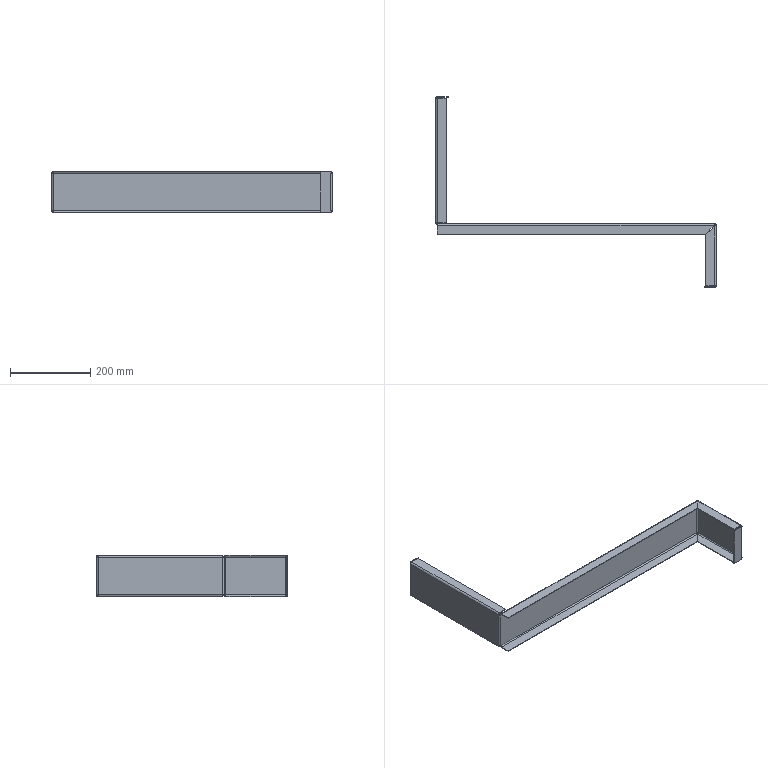Part | SolidWorks | features BaseBody 1 | 1 solid | 90 faces | box 701.5 x 477 x 103 mm | volume 268685 mm3 | plane 66 | cylinder 20 | spline 4 | commonest cylinder face diameters 6 x10 9 x10